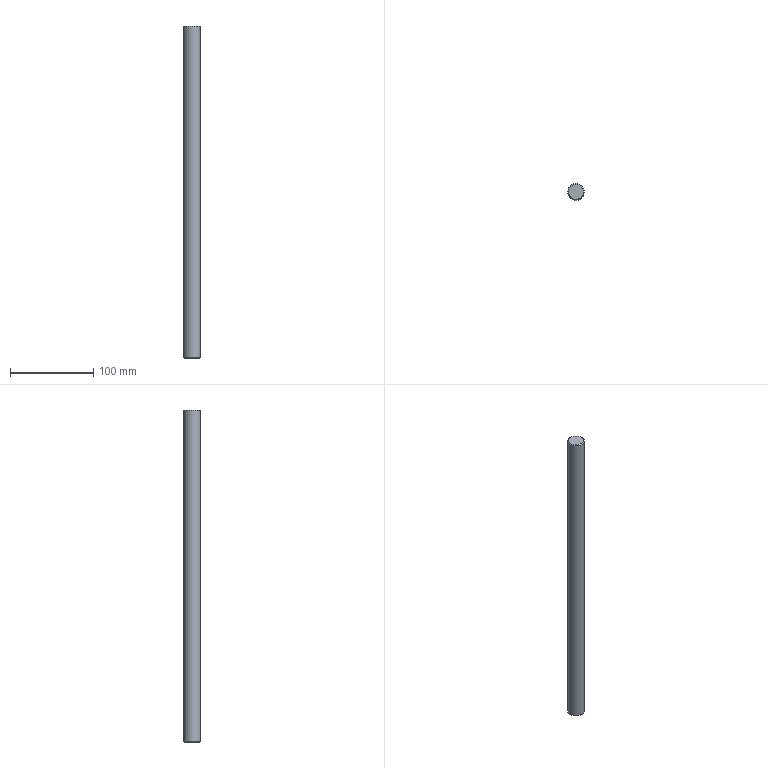Part | NX | features 001 2 | 1 solid | 5 faces | box 20 x 20 x 400 mm | volume 125603 mm3 | plane 2 | cone 2 | cylinder 1 | commonest cylinder face diameters 20 x1
STEP:
#1=CARTESIAN_POINT('',(84.691,17.319,-412.));
#2=VERTEX_POINT('',#1);
#3=CARTESIAN_POINT('',(80.,25.,-412.));
#4=DIRECTION('',(0.,0.,-1.));
#5=DIRECTION('',(0.5212,-0.8534,0.));
#6=AXIS2_PLACEMENT_3D('',#3,#4,#5);
#7=CIRCLE('',#6,9.);
#8=EDGE_CURVE('',#2,#2,#7,.T.);
#9=ORIENTED_EDGE('',*,*,#8,.T.);
#10=EDGE_LOOP('',(#9));
#11=FACE_BOUND('',#10,.T.);
#12=CARTESIAN_POINT('',(80.,25.,-412.));
#13=DIRECTION('',(0.,0.,1.));
#14=DIRECTION('',(-0.5212,0.8534,0.));
#15=AXIS2_PLACEMENT_3D('',#12,#13,#14);
#16=PLANE('',#15);
#17=ADVANCED_FACE('',(#11),#16,.F.);
#18=CARTESIAN_POINT('',(74.788,33.534,-411.));
#19=VERTEX_POINT('',#18);
#20=CARTESIAN_POINT('',(80.,25.,-411.));
#21=DIRECTION('',(0.,0.,-1.));
#22=DIRECTION('',(-0.5212,0.8534,0.));
#23=AXIS2_PLACEMENT_3D('',#20,#21,#22);
#24=CIRCLE('',#23,10.);
#25=EDGE_CURVE('',#19,#19,#24,.T.);
#26=ORIENTED_EDGE('',*,*,#25,.T.);
#27=EDGE_LOOP('',(#26));
#28=FACE_BOUND('',#27,.T.);
#29=ORIENTED_EDGE('',*,*,#8,.F.);
#30=EDGE_LOOP('',(#29));
#31=FACE_BOUND('',#30,.T.);
#32=CARTESIAN_POINT('',(80.,25.,-412.34));
#33=DIRECTION('',(0.,0.,1.));
#34=DIRECTION('',(-0.5212,0.8534,0.));
#35=AXIS2_PLACEMENT_3D('',#32,#33,#34);
#36=CONICAL_SURFACE('',#35,8.66,0.7854);
#37=ADVANCED_FACE('',(#28,#31),#36,.T.);
#38=ORIENTED_EDGE('',*,*,#25,.F.);
#39=EDGE_LOOP('',(#38));
#40=FACE_BOUND('',#39,.T.);
#41=CARTESIAN_POINT('',(74.788,33.534,-13.));
#42=VERTEX_POINT('',#41);
#43=CARTESIAN_POINT('',(80.,25.,-13.));
#44=DIRECTION('',(0.,0.,1.));
#45=DIRECTION('',(-0.5212,0.8534,0.));
#46=AXIS2_PLACEMENT_3D('',#43,#44,#45);
#47=CIRCLE('',#46,10.);
#48=EDGE_CURVE('',#42,#42,#47,.T.);
#49=ORIENTED_EDGE('',*,*,#48,.F.);
#50=EDGE_LOOP('',(#49));
#51=FACE_BOUND('',#50,.T.);
#52=CARTESIAN_POINT('',(80.,25.,-12.));
#53=DIRECTION('',(0.,0.,-1.));
#54=DIRECTION('',(0.5212,-0.8534,0.));
#55=AXIS2_PLACEMENT_3D('',#52,#53,#54);
#56=CYLINDRICAL_SURFACE('',#55,10.);
#57=ADVANCED_FACE('',(#40,#51),#56,.T.);
#58=CARTESIAN_POINT('',(75.309,32.681,-12.));
#59=VERTEX_POINT('',#58);
#60=CARTESIAN_POINT('',(80.,25.,-12.));
#61=DIRECTION('',(0.,0.,1.));
#62=DIRECTION('',(-0.5212,0.8534,0.));
#63=AXIS2_PLACEMENT_3D('',#60,#61,#62);
#64=CIRCLE('',#63,9.);
#65=EDGE_CURVE('',#59,#59,#64,.T.);
#66=ORIENTED_EDGE('',*,*,#65,.T.);
#67=EDGE_LOOP('',(#66));
#68=FACE_BOUND('',#67,.T.);
#69=CARTESIAN_POINT('',(80.,25.,-12.));
#70=DIRECTION('',(0.,0.,1.));
#71=DIRECTION('',(-0.5212,0.8534,0.));
#72=AXIS2_PLACEMENT_3D('',#69,#70,#71);
#73=PLANE('',#72);
#74=ADVANCED_FACE('',(#68),#73,.T.);
#75=ORIENTED_EDGE('',*,*,#65,.F.);
#76=EDGE_LOOP('',(#75));
#77=FACE_BOUND('',#76,.T.);
#78=ORIENTED_EDGE('',*,*,#48,.T.);
#79=EDGE_LOOP('',(#78));
#80=FACE_BOUND('',#79,.T.);
#81=CARTESIAN_POINT('',(80.,25.,-11.66));
#82=DIRECTION('',(0.,0.,-1.));
#83=DIRECTION('',(0.5212,-0.8534,0.));
#84=AXIS2_PLACEMENT_3D('',#81,#82,#83);
#85=CONICAL_SURFACE('',#84,8.66,0.7854);
#86=ADVANCED_FACE('',(#77,#80),#85,.T.);
#87=CLOSED_SHELL('',(#17,#37,#57,#74,#86));
#88=MANIFOLD_SOLID_BREP('',#87);
#89=(LENGTH_UNIT()NAMED_UNIT(*)SI_UNIT(.MILLI.,.METRE.));
#90=UNCERTAINTY_MEASURE_WITH_UNIT(LENGTH_MEASURE(0.00001),#89,'','');
#91=(NAMED_UNIT(*)PLANE_ANGLE_UNIT()SI_UNIT($,.RADIAN.));
#92=(NAMED_UNIT(*)SI_UNIT($,.STERADIAN.)SOLID_ANGLE_UNIT());
#93=(GEOMETRIC_REPRESENTATION_CONTEXT(3)GLOBAL_UNCERTAINTY_ASSIGNED_CONTEXT((#90))GLOBAL_UNIT_ASSIGNED_CONTEXT((#89,#91,#92))REPRESENTATION_CONTEXT('',''));
#94=ADVANCED_BREP_SHAPE_REPRESENTATION('',(#88),#93);